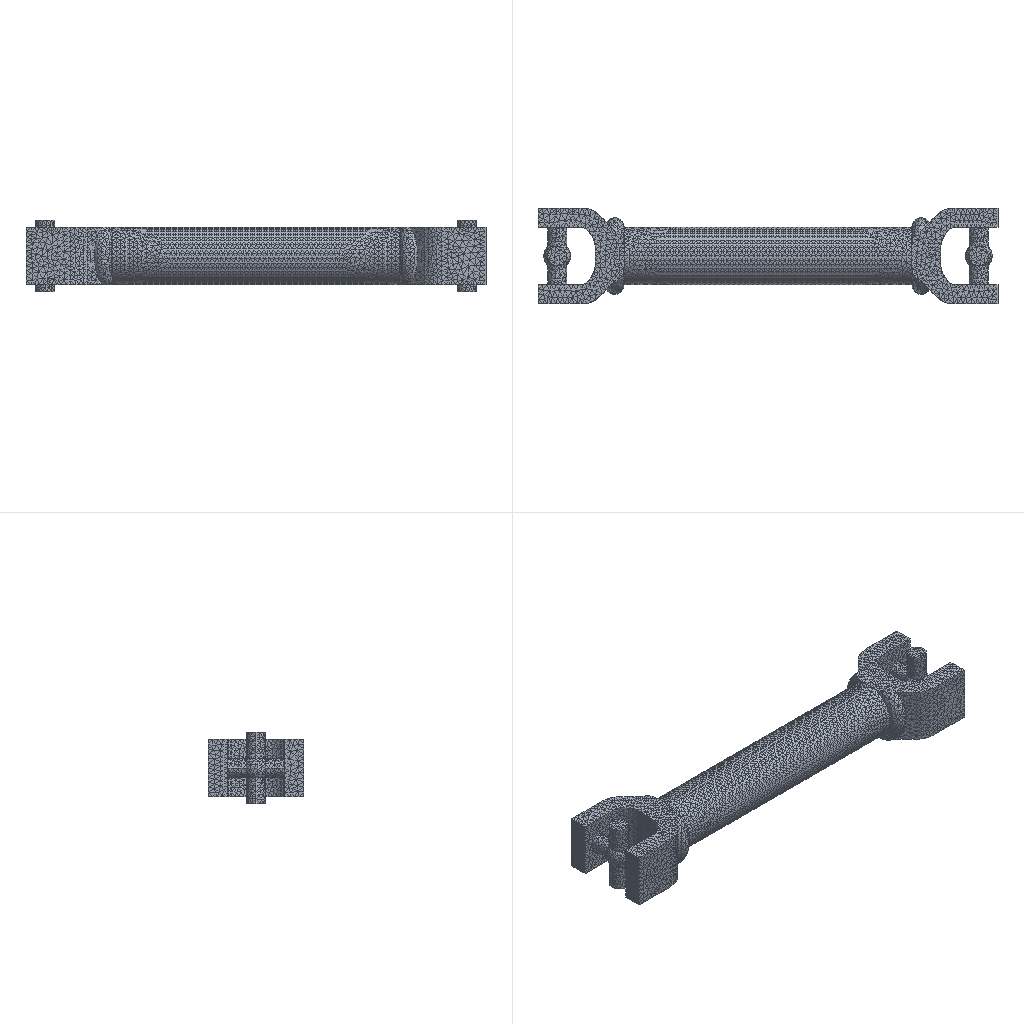Simulation study | ansys workbench
Set-up summary:
category,name,step,type,value,unit,region
solver,ansys_workbench
units,mm-N-s-tonne (MPa),,stated,"/units,MPA"
analysis,LS1,,static
load_step,LS1,LS1,static,nsubst=1; time=1
mesh,nodes,,,90917
mesh,elements,,,60202
element_type,SOLID187,,,58650
element_type,CONTA174,,,832
element_type,TARGE170,,,720
material,?,,E,240000,tonne s^-2 mm^-1
material,?,,nu,0.3
material,?,,density,6.9e-09,tonne mm^-3
material,16Mn?,,E,210000,tonne s^-2 mm^-1
material,16Mn?,,nu,0.3
material,16Mn?,,density,7.9e-09,tonne mm^-3
load,,LS1,moment,"1.1458e+06 [dir=(1, 0, 0) n=3]",,all
bc,,LS1,fixed,"[dofs=ROTX,ROTY,ROTZ,UX,UY,UZ n=6]",,node list
contact,Contact Region,,bonded (always),element=CONTA174
contact,Contact Region 2,,bonded (always),element=CONTA174
contact,contact 3,,bonded (always),element=CONTA174
contact,contact 4,,bonded (always),element=CONTA174
named_set,REMOTEDISPALL,,node,1
Ansys APDL input file, long lists of numbers shortened:
/batch
/config,noeldb,1     ! force off writing results to database
*get,_wallstrt,active,,time,wall
! ANSYS input file written by Workbench version 2021 R1
! File used for geometry attach:
/title,______--____ (B5)
! ****** Begin Custom Load Command Snippet ******
/COM, ACT Extensions:
/COM,     LSDYNA, 2021.1
/COM,
! ****** End   Custom Load Command Snippet ******
*DIM,_wb_ProjectScratch_dir,string,248
_wb_ProjectScratch_dir(1) = ''
*DIM,_wb_SolverFiles_dir,string,248
_wb_SolverFiles_dir(1) = ''
*DIM,_wb_userfiles_dir,string,248
_wb_userfiles_dir(1) = ''
/com,--- Data in consistent NMM units. See Solving Units in the help system for more information.
/units,MPA
/nopr
/wb,file,start              !  signify a WB generated input file
/prep7
! Turn off shape checking because checks already performed inside WB mesher.
! See help system for more information.
SHPP,OFF,,NOWARN
/nolist
etcon,set             ! allow ANSYS to choose best KEYOP's for 180x elements, resets any applicable keyopt to MAPDL defaults
/com,*********** Nodes for the whole assembly ***********
nblock,3,,100006
(1i9,3e20.9e3)
        1     7.600000000E+02    -2.000000000E+01     0.000000000E+00
! (90914 more lines like these left out)
-1
/com,*********** Nodes for all Remote Points ***********
nblock,3
(1i9,3e20.9e3)
    90916     7.400000000E+02     1.554312234E-14    -5.712370230E-07
    90917    -1.400000000E+02     1.402403685E-14    -1.421085472E-14
-1
/wb,elem,start            !  set before creation of elements
/com,*********** Elements for Body 1 "______|____2" ***********
et,1,187
eblock,19,solid,,52806
(19i9)
        1        1        1        1        0        0        0        0       10        0     5845    15480    21320    15698    17453    58957    61010    58952    58954
! (105611 more lines like these left out)
-1
/com,*********** Elements for Body 2 "______-0|____4" ***********
et,2,187
eblock,19,solid,,2922
(19i9)
        2        2        2        2        0        0        0        0       10        0     2923     5070     5085     5619     5377     6980     7061     6983     6981
! (5843 more lines like these left out)
-1
/com,*********** Elements for Body 3 "______-0|____4[2]" ***********
et,3,187
eblock,19,solid,,2922
(19i9)
        3        3        3        3        0        0        0        0       10        0        1      199      214      748      506     2109     2190     2112     2110
! (5843 more lines like these left out)
-1
/wb,elem,end               !  done creating elements
/com,*********** Send User Defined Coordinate System(s) ***********
csys,0
toffst,273.15,  ! Temperature offset from absolute zero
/com,*********** Set Reference Temperature ***********
tref,22.
/wb,mat,start              !  starting to send materials
/com,*********** Send Materials ***********
MP,DENS,1,6.9e-09,	! tonne mm^-3
MP,EX,1,240000,	! tonne s^-2 mm^-1
MP,NUXY,1,0.3,
MP,DENS,2,7.9e-09,	! tonne mm^-3
MP,EX,2,210000,	! tonne s^-2 mm^-1
MP,NUXY,2,0.3,
MP,DENS,3,7.9e-09,	! tonne mm^-3
MP,EX,3,210000,	! tonne s^-2 mm^-1
MP,NUXY,3,0.3,
/wb,mat,end                !  done sending materials
!************************* Model Summary ********************
!______|____2,	碳纤维合金钢,	matid,	1
!______-0|____4,	16Mn低合金钢,	matid,	2
!______-0|____4[2],	16Mn低合金钢,	matid,	3
!************************* End Model Summary ********************
! get the diagonal of the bounding box. Needed later for other things
*get,_xmin,node,,mnloc,x
*get,_ymin,node,,mnloc,y
*get,_zmin,node,,mnloc,z
*get,_xmax,node,,mxloc,x
*get,_ymax,node,,mxloc,y
*get,_zmax,node,,mxloc,z
_ASMDIAG=(_xmax-_xmin)*(_xmax-_xmin)+(_ymax-_ymin)*(_ymax-_ymin)+(_zmax-_zmin)*(_zmax-_zmin)
_ASMDIAG=SQRT(_ASMDIAG)
/wb,contact,start          !  starting to send contact
/com,*********** Create Contact "接触区域" ***********
/com,            Real Constant Set For Above Contact Is 5 & 4
*set,tid,5
*set,cid,4
r,tid
r,cid
et,tid,170
et,cid,174
eblock,10,,,160
(15i9)
    70893        5        5        5        0     9779     9788     9781     9781    21636    21646     9781    21635
! (159 more lines like these left out)
-1
eblock,10,,,160
(15i9)
    71053        4        4        4        0     9779     9788     9781     9781    21636    21646     9781    21635
! (159 more lines like these left out)
-1
eblock,10,,,200
(15i9)
    71213        4        5        4        0     4877     4884     4882     4882     5669     5706     4882     5668
! (199 more lines like these left out)
-1
eblock,10,,,200
(15i9)
    71413        5        4        5        0     4877     4884     4882     4882     5669     5706     4882     5668
! (199 more lines like these left out)
-1
keyo,cid,8,2               ! auto create asymmetric contact (from Program Controlled setting)
keyo,cid,10,0              ! adjust contact stiffness each NR iteration (from Program Controlled setting)
keyo,cid,12,5              ! bonded always
keyo,cid,18,1              ! small sliding turned on by application
keyo,cid,2,0               ! augmented Lagrange (from Program Controlled setting)
keyo,cid,4,0               ! on Gauss point (from Program Controlled setting)
keyo,cid,9,1               ! ignore initial gaps/penetration
keyo,cid,7,0               ! No Prediction
rmod,tid,3,10.      ! FKN
rmod,tid,5,0.       ! ICONT
rmod,tid,6,0.       ! PINB
rmod,tid,10,0.      ! CNOF
rmod,tid,12,0.      ! FKT
rmod,tid,36,31      ! WB DSID
rmod,cid,3,10.      ! FKN
rmod,cid,5,0.       ! ICONT
rmod,cid,6,0.       ! PINB
rmod,cid,10,0.      ! CNOF
rmod,cid,12,0.      ! FKT
rmod,cid,36,31      ! WB DSID
/com,*********** Create Contact "接触区域 2" ***********
/com,            Real Constant Set For Above Contact Is 7 & 6
*set,tid,7
*set,cid,6
r,tid
r,cid
et,tid,170
et,cid,174
eblock,10,,,160
(15i9)
    71613        7        7        7        0     9744     9752     9750     9750    21332    21399     9750    21331
! (159 more lines like these left out)
-1
eblock,10,,,160
(15i9)
    71773        6        6        6        0     9744     9752     9750     9750    21332    21399     9750    21331
! (159 more lines like these left out)
-1
eblock,10,,,200
(15i9)
    71933        6        7        6        0       57       55       64       64     1172     1173       64     1181
! (199 more lines like these left out)
-1
eblock,10,,,200
(15i9)
    72133        7        6        7        0       57       55       64       64     1172     1173       64     1181
! (199 more lines like these left out)
-1
keyo,cid,8,2               ! auto create asymmetric contact (from Program Controlled setting)
keyo,cid,10,0              ! adjust contact stiffness each NR iteration (from Program Controlled setting)
keyo,cid,12,5              ! bonded always
keyo,cid,18,1              ! small sliding turned on by application
keyo,cid,2,0               ! augmented Lagrange (from Program Controlled setting)
keyo,cid,4,0               ! on Gauss point (from Program Controlled setting)
keyo,cid,9,1               ! ignore initial gaps/penetration
keyo,cid,7,0               ! No Prediction
rmod,tid,3,10.      ! FKN
rmod,tid,5,0.       ! ICONT
rmod,tid,6,0.       ! PINB
rmod,tid,10,0.      ! CNOF
rmod,tid,12,0.      ! FKT
rmod,tid,36,34      ! WB DSID
rmod,cid,3,10.      ! FKN
rmod,cid,5,0.       ! ICONT
rmod,cid,6,0.       ! PINB
rmod,cid,10,0.      ! CNOF
rmod,cid,12,0.      ! FKT
rmod,cid,36,34      ! WB DSID
nsel,all
esel,all
/wb,contact,end            !  done creating contacts
/golist
/wb,load,start             !  starting to send loads
/com,*********** Create Remote Point "内部远程点" ***********
! -------- Remote Point Used by "远程位移" --------
*set,tid,9
*set,cid,8
et,cid,174
et,tid,170
keyo,tid,2,1               ! Don't fix the pilot node
keyo,tid,4,111111
keyo,cid,12,5              ! Bonded Contact
keyo,cid,4,1               ! Deformable RBE3 style load
keyo,cid,2,2               ! MPC style contact
eblock,10,,,56
(15i9)
    72333        8        8        8        0      148      437      149      149     1846     1851      149     1843
! (55 more lines like these left out)
-1
*set,_npilot,90916
_npilot44=_npilot
type,tid
mat ,cid
real,cid
tshape,pilo
en,72389,_npilot
tshape
/com,*********** Create Remote Point "内部远程点 2" ***********
! -------- Remote Point Used by "力矩" --------
*set,tid,11
*set,cid,10
et,cid,174
et,tid,170
keyo,tid,2,1               ! Don't fix the pilot node
keyo,tid,4,111111
keyo,cid,12,5              ! Bonded Contact
keyo,cid,4,1               ! Deformable RBE3 style load
keyo,cid,2,2               ! MPC style contact
eblock,10,,,56
(15i9)
    72390       10       10       10        0     5019     5308     5020     5020     6717     6722     5020     6714
! (55 more lines like these left out)
-1
*set,_npilot,90917
_npilot47=_npilot
type,tid
mat ,cid
real,cid
tshape,pilo
en,72446,_npilot
tshape
/com,*********** Construct Moment Using Remote Attachment ***********
/com,*********** Construct Remote Displacement ***********
/COM,*** Create a component for all remote displacements ***
CMBLOCK,REMOTEDISPALL,NODE,        1
(8i10)
     90916
/gst,on,on
fini
*get,_numnode,node,0,count
*get,_numelem,elem,0,count
*get, _MAXELEMNUM, elem, 0, NUM, MAX
*get, _MAXNODENUM, node, 0, NUM, MAX
*get, _MAXELEMTYPE, etyp, 0, NUM, MAX
*get, _MAXREALCONST, real, 0, NUM, MAX
/go
/wb,load,end               !  done creating loads
/com,--- Number of total nodes = %_numnode%
/com,--- Number of contact elements = 1552
/com,--- Number of spring elements = 0
/com,--- Number of bearing elements = 0
/com,--- Number of solid elements = 58650
/com,--- Number of condensed parts = 0
/com,--- Number of total elements = %_numelem%
*get,_wallbsol,active,,time,wall
/com,****************************************************************************
/com,*************************    SOLUTION       ********************************
/com,****************************************************************************
/solu
antype,0                   ! static analysis
_thickRatio=  1     ! Ratio of thick parts in the model
eqsl,pcg,1e-8,,,,,,1
cntr,print,1               ! print out contact info and also make no initial contact an error
dmpoption,emat,no             ! Don't combine emat file for DANSYS
dmpoption,esav,no             ! Don't combine esav file for DANSYS
nldiag,cont,iter           ! print out contact info each equilibrium iteration
rescontrol,,none                 ! Do not keep any restart files
/com,****************************************************
/com,******************* SOLVE FOR LS 1 OF 1 ****************
nsel,s,node,,90917
f,all,mx,1145800.
f,all,my,0.
f,all,mz,0.
nsel,all
d,90916,ux,0.
d,90916,uy,0.
d,90916,uz,0.
d,90916,rotx,0.
d,90916,roty,0.
d,90916,rotz,0.
/nopr
/gopr
/nolist
nsub,1,1,1
time,1.
outres,erase
outres,all,none
outres,nsol,all,
outres,rsol,all
outres,eangl,all
outres,etmp,all
outres,veng,all
outres,strs,all,
outres,epel,all,
outres,eppl,all,
outres,cont,all,
! *********** WB SOLVE COMMAND ***********
! check interactive state
*get,ANSINTER_,active,,int
*if,ANSINTER_,ne,0,then
/eof
*endif
solve
/com *************** Write FE CONNECTORS *********
CEWRITE,file,ce,,INTE
/com,****************************************************
/com,*************** FINISHED SOLVE FOR LS 1 *************
*get,_wallasol,active,,time,wall
/nopr
*get,_numnode,node,0,count
*get,_numelem,elem,0,count
*get, _MAXELEMNUM, elem, 0, NUM, MAX
*get, _MAXNODENUM, node, 0, NUM, MAX,,,INTERNAL
*get, _MAXELEMTYPE, etyp, 0, NUM, MAX
*get, _MAXREALCONST, real, 0, NUM, MAX
/gopr
*get,_PCGITER,active,,solu,cgiter
/post1
xmlo,ENCODING,ISO-8859-1
xmlo,parm
/xml,parm,xml
fini
/gopr
*get,_walldone,active,,time,wall
_preptime=(_wallbsol-_wallstrt)*3600
_solvtime=(_wallasol-_wallbsol)*3600
_posttime=(_walldone-_wallasol)*3600
_totaltim=(_walldone-_wallstrt)*3600
*get,_dlbratio,active,0,solu,dlbr
*get,_combtime,active,0,solu,comb
/com,--- Total number of nodes = %_numnode%
/com,--- Total number of elements = %_numelem%
/com,--- Element load balance ratio = %_dlbratio%
/com,--- Time to combine distributed files = %_combtime%
/wb,file,end               ! done with WB generated input
Results summary:
result,analyses[0].index,,,1
result,analyses[0].system,,,SYS-1
result,analyses[0].deck,,,deck.dat
result,analyses[0].solve_status,,,completed
result,analyses[0].analysis_type,,,static
result,analyses[0].physics,,,mechanical
result,analyses[0].unit_system,,,"NMM: mm, ton, N, s, mV, mA, degC"
result,analyses[0].n_sets,,,1
result,analyses[0].load_steps[0].set,set=1,,1
result,analyses[0].load_steps[0].time_or_freq,set=1,,1
result,analyses[0].load_steps[0].max_displacement_magnitude,set=1,,0.1602
result,analyses[0].load_steps[0].max_von_mises_nodal,set=1,,90.552
result,analyses[0].load_steps[0].reaction_force_sum_xyz[1],set=1,,0.0075
result,analyses[0].load_steps[0].reaction_force_sum_xyz[2],set=1,,-0.001522
result,analyses[0].load_steps[0].reaction_force_sum_xyz[3],set=1,,-0.001826
result,geometry_export[0][0],,,.step
result,geometry_export[0][1],,,ok
result,geometry_export[0][2],,,3